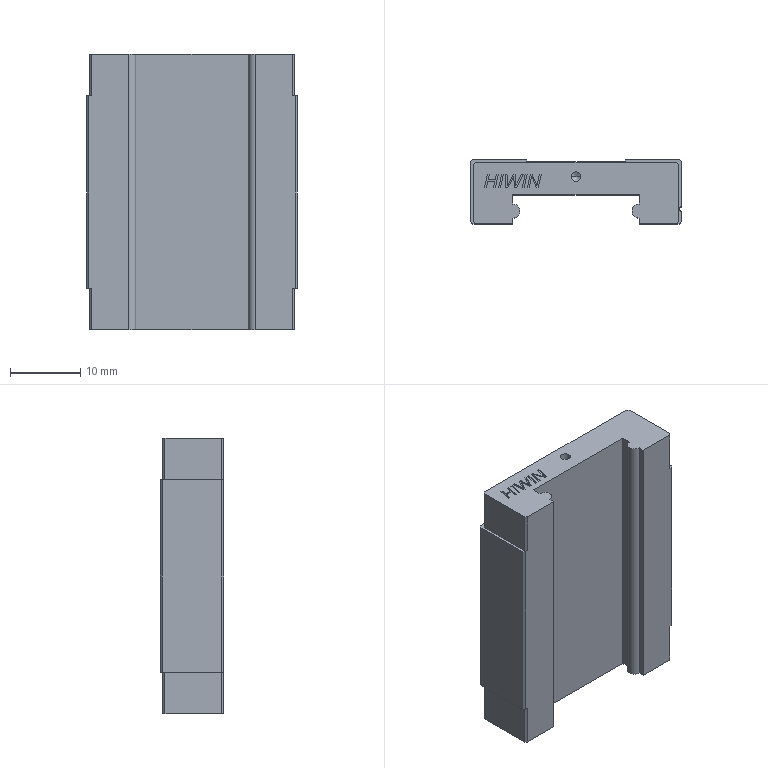Part | SolidWorks | features BaseBody 1 | 1 solid | 203 faces | box 30 x 9.1 x 39.3 mm | volume 7510 mm3 | plane 116 | spline 58 | cylinder 17 | cone 12 | commonest cylinder face diameters 3 x8 1.4 x4 2 x3 0.6 x2